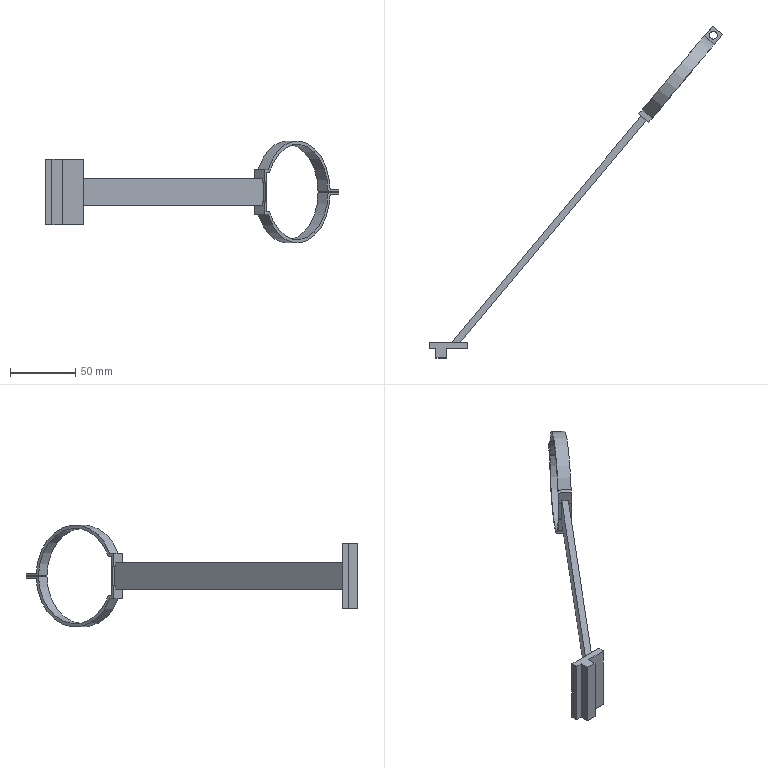Part | SolidWorks | features ICE 7, MirrorPattern 2, BossThin 1, Extrusion 1 | 1 solid | 43 faces | box 224.292 x 253.925 x 78 mm | volume 38659 mm3 | plane 35 | cylinder 8 | commonest cylinder face diameters 6 x4 73 x2 78 x2
STEP:
#1=CARTESIAN_POINT('',(195.164,232.208,2.));
#2=VERTEX_POINT('',#1);
#3=CARTESIAN_POINT('',(201.164,232.208,2.));
#4=VERTEX_POINT('',#3);
#5=CARTESIAN_POINT('',(198.164,232.208,2.));
#6=DIRECTION('',(0.,0.,1.));
#7=DIRECTION('',(1.,0.,0.));
#8=AXIS2_PLACEMENT_3D('',#5,#6,#7);
#9=CIRCLE('',#8,3.);
#10=EDGE_CURVE('',#2,#4,#9,.T.);
#11=ORIENTED_EDGE('',*,*,#10,.T.);
#12=CARTESIAN_POINT('',(201.164,232.208,0.5));
#13=VERTEX_POINT('',#12);
#14=CARTESIAN_POINT('',(201.164,232.208,39.));
#15=DIRECTION('',(0.,0.,-1.));
#16=VECTOR('',#15,1000.);
#17=LINE('',#14,#16);
#18=EDGE_CURVE('',#4,#13,#17,.T.);
#19=ORIENTED_EDGE('',*,*,#18,.T.);
#20=CARTESIAN_POINT('',(195.164,232.208,0.5));
#21=VERTEX_POINT('',#20);
#22=CARTESIAN_POINT('',(198.164,232.208,0.5));
#23=DIRECTION('',(0.,0.,1.));
#24=DIRECTION('',(1.,0.,0.));
#25=AXIS2_PLACEMENT_3D('',#22,#23,#24);
#26=CIRCLE('',#25,3.);
#27=EDGE_CURVE('',#21,#13,#26,.T.);
#28=ORIENTED_EDGE('',*,*,#27,.F.);
#29=CARTESIAN_POINT('',(195.164,232.208,39.));
#30=DIRECTION('',(0.,0.,-1.));
#31=VECTOR('',#30,1000.);
#32=LINE('',#29,#31);
#33=EDGE_CURVE('',#2,#21,#32,.T.);
#34=ORIENTED_EDGE('',*,*,#33,.F.);
#35=EDGE_LOOP('',(#11,#19,#28,#34));
#36=FACE_OUTER_BOUND('',#35,.T.);
#37=CARTESIAN_POINT('',(198.164,232.208,39.));
#38=DIRECTION('',(0.,0.,-1.));
#39=DIRECTION('',(-1.,0.,0.));
#40=AXIS2_PLACEMENT_3D('',#37,#38,#39);
#41=CYLINDRICAL_SURFACE('',#40,3.);
#42=ADVANCED_FACE('',(#36),#41,.F.);
#43=CARTESIAN_POINT('',(201.164,232.208,-0.5));
#44=VERTEX_POINT('',#43);
#45=CARTESIAN_POINT('',(195.164,232.208,-0.5));
#46=VERTEX_POINT('',#45);
#47=CARTESIAN_POINT('',(198.164,232.208,-0.5));
#48=DIRECTION('',(0.,0.,-1.));
#49=DIRECTION('',(-1.,0.,0.));
#50=AXIS2_PLACEMENT_3D('',#47,#48,#49);
#51=CIRCLE('',#50,3.);
#52=EDGE_CURVE('',#44,#46,#51,.T.);
#53=ORIENTED_EDGE('',*,*,#52,.F.);
#54=CARTESIAN_POINT('',(201.164,232.208,-2.));
#55=VERTEX_POINT('',#54);
#56=CARTESIAN_POINT('',(201.164,232.208,39.));
#57=DIRECTION('',(0.,0.,-1.));
#58=VECTOR('',#57,1000.);
#59=LINE('',#56,#58);
#60=EDGE_CURVE('',#44,#55,#59,.T.);
#61=ORIENTED_EDGE('',*,*,#60,.T.);
#62=CARTESIAN_POINT('',(195.164,232.208,-2.));
#63=VERTEX_POINT('',#62);
#64=CARTESIAN_POINT('',(198.164,232.208,-2.));
#65=DIRECTION('',(0.,0.,1.));
#66=DIRECTION('',(1.,0.,0.));
#67=AXIS2_PLACEMENT_3D('',#64,#65,#66);
#68=CIRCLE('',#67,3.);
#69=EDGE_CURVE('',#63,#55,#68,.T.);
#70=ORIENTED_EDGE('',*,*,#69,.F.);
#71=CARTESIAN_POINT('',(195.164,232.208,39.));
#72=DIRECTION('',(0.,0.,-1.));
#73=VECTOR('',#72,1000.);
#74=LINE('',#71,#73);
#75=EDGE_CURVE('',#46,#63,#74,.T.);
#76=ORIENTED_EDGE('',*,*,#75,.F.);
#77=EDGE_LOOP('',(#53,#61,#70,#76));
#78=FACE_OUTER_BOUND('',#77,.T.);
#79=CARTESIAN_POINT('',(198.164,232.208,39.));
#80=DIRECTION('',(0.,0.,-1.));
#81=DIRECTION('',(-1.,0.,0.));
#82=AXIS2_PLACEMENT_3D('',#79,#80,#81);
#83=CYLINDRICAL_SURFACE('',#82,3.);
#84=ADVANCED_FACE('',(#78),#83,.F.);
#85=CARTESIAN_POINT('',(143.02,170.445,10.));
#86=VERTEX_POINT('',#85);
#87=CARTESIAN_POINT('',(-2.232,-2.66,10.));
#88=VERTEX_POINT('',#87);
#89=CARTESIAN_POINT('',(0.,0.,10.));
#90=DIRECTION('',(-0.6428,-0.766,0.));
#91=VECTOR('',#90,1000.);
#92=LINE('',#89,#91);
#93=EDGE_CURVE('',#86,#88,#92,.T.);
#94=ORIENTED_EDGE('',*,*,#93,.T.);
#95=CARTESIAN_POINT('',(4.295,-2.66,10.));
#96=VERTEX_POINT('',#95);
#97=CARTESIAN_POINT('',(4.295,-2.66,10.));
#98=DIRECTION('',(-1.,0.,0.));
#99=VECTOR('',#98,1000.);
#100=LINE('',#97,#99);
#101=EDGE_CURVE('',#96,#88,#100,.T.);
#102=ORIENTED_EDGE('',*,*,#101,.F.);
#103=CARTESIAN_POINT('',(146.85,167.231,10.));
#104=VERTEX_POINT('',#103);
#105=CARTESIAN_POINT('',(4.295,-2.66,10.));
#106=DIRECTION('',(0.6428,0.766,0.));
#107=VECTOR('',#106,1000.);
#108=LINE('',#105,#107);
#109=EDGE_CURVE('',#96,#104,#108,.T.);
#110=ORIENTED_EDGE('',*,*,#109,.T.);
#111=CARTESIAN_POINT('',(143.02,170.445,10.));
#112=DIRECTION('',(0.766,-0.6428,0.));
#113=VECTOR('',#112,1000.);
#114=LINE('',#111,#113);
#115=EDGE_CURVE('',#86,#104,#114,.T.);
#116=ORIENTED_EDGE('',*,*,#115,.F.);
#117=EDGE_LOOP('',(#94,#102,#110,#116));
#118=FACE_OUTER_BOUND('',#117,.T.);
#119=CARTESIAN_POINT('',(0.,0.,10.));
#120=DIRECTION('',(0.,0.,1.));
#121=DIRECTION('',(1.,0.,0.));
#122=AXIS2_PLACEMENT_3D('',#119,#120,#121);
#123=PLANE('',#122);
#124=ADVANCED_FACE('',(#118),#123,.T.);
#125=CARTESIAN_POINT('',(191.045,231.567,-2.));
#126=VERTEX_POINT('',#125);
#127=CARTESIAN_POINT('',(143.606,175.032,-17.5));
#128=VERTEX_POINT('',#127);
#129=CARTESIAN_POINT('',(166.009,201.731,0.));
#130=DIRECTION('',(-0.766,0.6428,0.));
#131=DIRECTION('',(0.,0.,1.));
#132=AXIS2_PLACEMENT_3D('',#129,#130,#131);
#133=CIRCLE('',#132,39.);
#134=EDGE_CURVE('',#126,#128,#133,.T.);
#135=ORIENTED_EDGE('',*,*,#134,.F.);
#136=CARTESIAN_POINT('',(198.705,225.139,-2.));
#137=VERTEX_POINT('',#136);
#138=CARTESIAN_POINT('',(198.705,225.139,-2.));
#139=DIRECTION('',(-0.766,0.6428,0.));
#140=VECTOR('',#139,1000.);
#141=LINE('',#138,#140);
#142=EDGE_CURVE('',#137,#126,#141,.T.);
#143=ORIENTED_EDGE('',*,*,#142,.F.);
#144=CARTESIAN_POINT('',(151.266,168.604,-17.5));
#145=VERTEX_POINT('',#144);
#146=CARTESIAN_POINT('',(173.669,195.303,0.));
#147=DIRECTION('',(-0.766,0.6428,0.));
#148=DIRECTION('',(0.,0.,1.));
#149=AXIS2_PLACEMENT_3D('',#146,#147,#148);
#150=CIRCLE('',#149,39.);
#151=EDGE_CURVE('',#137,#145,#150,.T.);
#152=ORIENTED_EDGE('',*,*,#151,.T.);
#153=CARTESIAN_POINT('',(151.266,168.604,-17.5));
#154=DIRECTION('',(-0.766,0.6428,0.));
#155=VECTOR('',#154,1000.);
#156=LINE('',#153,#155);
#157=EDGE_CURVE('',#145,#128,#156,.T.);
#158=ORIENTED_EDGE('',*,*,#157,.T.);
#159=EDGE_LOOP('',(#135,#143,#152,#158));
#160=FACE_OUTER_BOUND('',#159,.T.);
#161=CARTESIAN_POINT('',(173.669,195.303,0.));
#162=DIRECTION('',(-0.766,0.6428,0.));
#163=DIRECTION('',(-0.6428,-0.766,0.));
#164=AXIS2_PLACEMENT_3D('',#161,#162,#163);
#165=CYLINDRICAL_SURFACE('',#164,39.);
#166=ADVANCED_FACE('',(#160),#165,.T.);
#167=CARTESIAN_POINT('',(198.705,225.139,2.));
#168=VERTEX_POINT('',#167);
#169=CARTESIAN_POINT('',(191.045,231.567,2.));
#170=VERTEX_POINT('',#169);
#171=CARTESIAN_POINT('',(198.705,225.139,2.));
#172=DIRECTION('',(-0.766,0.6428,0.));
#173=VECTOR('',#172,1000.);
#174=LINE('',#171,#173);
#175=EDGE_CURVE('',#168,#170,#174,.T.);
#176=ORIENTED_EDGE('',*,*,#175,.T.);
#177=CARTESIAN_POINT('',(143.606,175.032,17.5));
#178=VERTEX_POINT('',#177);
#179=CARTESIAN_POINT('',(166.009,201.731,0.));
#180=DIRECTION('',(-0.766,0.6428,0.));
#181=DIRECTION('',(0.,0.,1.));
#182=AXIS2_PLACEMENT_3D('',#179,#180,#181);
#183=CIRCLE('',#182,39.);
#184=EDGE_CURVE('',#178,#170,#183,.T.);
#185=ORIENTED_EDGE('',*,*,#184,.F.);
#186=CARTESIAN_POINT('',(151.266,168.604,17.5));
#187=VERTEX_POINT('',#186);
#188=CARTESIAN_POINT('',(151.266,168.604,17.5));
#189=DIRECTION('',(-0.766,0.6428,0.));
#190=VECTOR('',#189,1000.);
#191=LINE('',#188,#190);
#192=EDGE_CURVE('',#187,#178,#191,.T.);
#193=ORIENTED_EDGE('',*,*,#192,.F.);
#194=CARTESIAN_POINT('',(173.669,195.303,0.));
#195=DIRECTION('',(-0.766,0.6428,0.));
#196=DIRECTION('',(0.,0.,1.));
#197=AXIS2_PLACEMENT_3D('',#194,#195,#196);
#198=CIRCLE('',#197,39.);
#199=EDGE_CURVE('',#187,#168,#198,.T.);
#200=ORIENTED_EDGE('',*,*,#199,.T.);
#201=EDGE_LOOP('',(#176,#185,#193,#200));
#202=FACE_OUTER_BOUND('',#201,.T.);
#203=CARTESIAN_POINT('',(173.669,195.303,0.));
#204=DIRECTION('',(-0.766,0.6428,0.));
#205=DIRECTION('',(-0.6428,-0.766,0.));
#206=AXIS2_PLACEMENT_3D('',#203,#204,#205);
#207=CYLINDRICAL_SURFACE('',#206,39.);
#208=ADVANCED_FACE('',(#202),#207,.T.);
#209=CARTESIAN_POINT('',(144.62,176.24,15.));
#210=VERTEX_POINT('',#209);
#211=CARTESIAN_POINT('',(189.468,229.689,0.5));
#212=VERTEX_POINT('',#211);
#213=CARTESIAN_POINT('',(166.009,201.731,0.));
#214=DIRECTION('',(-0.766,0.6428,0.));
#215=DIRECTION('',(-0.6428,-0.766,0.));
#216=AXIS2_PLACEMENT_3D('',#213,#214,#215);
#217=CIRCLE('',#216,36.5);
#218=EDGE_CURVE('',#210,#212,#217,.T.);
#219=ORIENTED_EDGE('',*,*,#218,.T.);
#220=CARTESIAN_POINT('',(197.129,223.261,0.5));
#221=VERTEX_POINT('',#220);
#222=CARTESIAN_POINT('',(197.129,223.261,0.5));
#223=DIRECTION('',(0.766,-0.6428,0.));
#224=VECTOR('',#223,1000.);
#225=LINE('',#222,#224);
#226=EDGE_CURVE('',#212,#221,#225,.T.);
#227=ORIENTED_EDGE('',*,*,#226,.T.);
#228=CARTESIAN_POINT('',(152.28,169.813,15.));
#229=VERTEX_POINT('',#228);
#230=CARTESIAN_POINT('',(173.669,195.303,0.));
#231=DIRECTION('',(-0.766,0.6428,0.));
#232=DIRECTION('',(-0.6428,-0.766,0.));
#233=AXIS2_PLACEMENT_3D('',#230,#231,#232);
#234=CIRCLE('',#233,36.5);
#235=EDGE_CURVE('',#229,#221,#234,.T.);
#236=ORIENTED_EDGE('',*,*,#235,.F.);
#237=CARTESIAN_POINT('',(152.28,169.813,15.));
#238=DIRECTION('',(-0.766,0.6428,0.));
#239=VECTOR('',#238,1000.);
#240=LINE('',#237,#239);
#241=EDGE_CURVE('',#229,#210,#240,.T.);
#242=ORIENTED_EDGE('',*,*,#241,.T.);
#243=EDGE_LOOP('',(#219,#227,#236,#242));
#244=FACE_OUTER_BOUND('',#243,.T.);
#245=CARTESIAN_POINT('',(173.669,195.303,0.));
#246=DIRECTION('',(-0.766,0.6428,0.));
#247=DIRECTION('',(-0.6428,-0.766,0.));
#248=AXIS2_PLACEMENT_3D('',#245,#246,#247);
#249=CYLINDRICAL_SURFACE('',#248,36.5);
#250=ADVANCED_FACE('',(#244),#249,.F.);
#251=CARTESIAN_POINT('',(-6.128,-7.66,25.));
#252=VERTEX_POINT('',#251);
#253=CARTESIAN_POINT('',(10.,-7.66,25.));
#254=VERTEX_POINT('',#253);
#255=CARTESIAN_POINT('',(-6.428,-7.66,25.));
#256=DIRECTION('',(1.,0.,0.));
#257=VECTOR('',#256,1000.);
#258=LINE('',#255,#257);
#259=EDGE_CURVE('',#252,#254,#258,.T.);
#260=ORIENTED_EDGE('',*,*,#259,.F.);
#261=CARTESIAN_POINT('',(-6.128,-7.66,-25.));
#262=VERTEX_POINT('',#261);
#263=CARTESIAN_POINT('',(-6.128,-7.66,45.723));
#264=DIRECTION('',(0.,0.,-1.));
#265=VECTOR('',#264,1000.);
#266=LINE('',#263,#265);
#267=EDGE_CURVE('',#252,#262,#266,.T.);
#268=ORIENTED_EDGE('',*,*,#267,.T.);
#269=CARTESIAN_POINT('',(10.,-7.66,-25.));
#270=VERTEX_POINT('',#269);
#271=CARTESIAN_POINT('',(-6.428,-7.66,-25.));
#272=DIRECTION('',(1.,0.,0.));
#273=VECTOR('',#272,1000.);
#274=LINE('',#271,#273);
#275=EDGE_CURVE('',#262,#270,#274,.T.);
#276=ORIENTED_EDGE('',*,*,#275,.T.);
#277=CARTESIAN_POINT('',(10.,-7.66,10.));
#278=DIRECTION('',(0.,0.,-1.));
#279=VECTOR('',#278,1000.);
#280=LINE('',#277,#279);
#281=EDGE_CURVE('',#254,#270,#280,.T.);
#282=ORIENTED_EDGE('',*,*,#281,.F.);
#283=EDGE_LOOP('',(#260,#268,#276,#282));
#284=FACE_OUTER_BOUND('',#283,.T.);
#285=CARTESIAN_POINT('',(-6.428,-7.66,10.));
#286=DIRECTION('',(0.,1.,0.));
#287=DIRECTION('',(0.,0.,1.));
#288=AXIS2_PLACEMENT_3D('',#285,#286,#287);
#289=PLANE('',#288);
#290=ADVANCED_FACE('',(#284),#289,.F.);
#291=CARTESIAN_POINT('',(-2.232,-2.66,-10.));
#292=VERTEX_POINT('',#291);
#293=CARTESIAN_POINT('',(-2.232,-2.66,45.723));
#294=DIRECTION('',(0.,0.,-1.));
#295=VECTOR('',#294,1000.);
#296=LINE('',#293,#295);
#297=EDGE_CURVE('',#88,#292,#296,.T.);
#298=ORIENTED_EDGE('',*,*,#297,.T.);
#299=CARTESIAN_POINT('',(4.295,-2.66,-10.));
#300=VERTEX_POINT('',#299);
#301=CARTESIAN_POINT('',(10.,-2.66,-10.));
#302=DIRECTION('',(-1.,0.,0.));
#303=VECTOR('',#302,1000.);
#304=LINE('',#301,#303);
#305=EDGE_CURVE('',#300,#292,#304,.T.);
#306=ORIENTED_EDGE('',*,*,#305,.F.);
#307=CARTESIAN_POINT('',(4.295,-2.66,10.));
#308=DIRECTION('',(0.,0.,-1.));
#309=VECTOR('',#308,1000.);
#310=LINE('',#307,#309);
#311=EDGE_CURVE('',#96,#300,#310,.T.);
#312=ORIENTED_EDGE('',*,*,#311,.F.);
#313=ORIENTED_EDGE('',*,*,#101,.T.);
#314=EDGE_LOOP('',(#298,#306,#312,#313));
#315=FACE_BOUND('',#314,.T.);
#316=CARTESIAN_POINT('',(10.,-2.66,-25.));
#317=VERTEX_POINT('',#316);
#318=CARTESIAN_POINT('',(-19.128,-2.66,-25.));
#319=VERTEX_POINT('',#318);
#320=CARTESIAN_POINT('',(4.295,-2.66,-25.));
#321=DIRECTION('',(-1.,0.,0.));
#322=VECTOR('',#321,1000.);
#323=LINE('',#320,#322);
#324=EDGE_CURVE('',#317,#319,#323,.T.);
#325=ORIENTED_EDGE('',*,*,#324,.T.);
#326=CARTESIAN_POINT('',(-19.128,-2.66,25.));
#327=VERTEX_POINT('',#326);
#328=CARTESIAN_POINT('',(-19.128,-2.66,45.723));
#329=DIRECTION('',(0.,0.,-1.));
#330=VECTOR('',#329,1000.);
#331=LINE('',#328,#330);
#332=EDGE_CURVE('',#327,#319,#331,.T.);
#333=ORIENTED_EDGE('',*,*,#332,.F.);
#334=CARTESIAN_POINT('',(10.,-2.66,25.));
#335=VERTEX_POINT('',#334);
#336=CARTESIAN_POINT('',(10.,-2.66,25.));
#337=DIRECTION('',(-1.,0.,0.));
#338=VECTOR('',#337,1000.);
#339=LINE('',#336,#338);
#340=EDGE_CURVE('',#335,#327,#339,.T.);
#341=ORIENTED_EDGE('',*,*,#340,.F.);
#342=CARTESIAN_POINT('',(10.,-2.66,10.));
#343=DIRECTION('',(0.,0.,-1.));
#344=VECTOR('',#343,1000.);
#345=LINE('',#342,#344);
#346=EDGE_CURVE('',#335,#317,#345,.T.);
#347=ORIENTED_EDGE('',*,*,#346,.T.);
#348=EDGE_LOOP('',(#325,#333,#341,#347));
#349=FACE_OUTER_BOUND('',#348,.T.);
#350=CARTESIAN_POINT('',(30.,-2.66,10.));
#351=DIRECTION('',(0.,-1.,0.));
#352=DIRECTION('',(1.,0.,0.));
#353=AXIS2_PLACEMENT_3D('',#350,#351,#352);
#354=PLANE('',#353);
#355=ADVANCED_FACE('',(#315,#349),#354,.F.);
#356=CARTESIAN_POINT('',(147.493,167.997,7.5));
#357=VERTEX_POINT('',#356);
#358=CARTESIAN_POINT('',(146.85,167.231,7.5));
#359=VERTEX_POINT('',#358);
#360=CARTESIAN_POINT('',(149.1,169.912,7.5));
#361=DIRECTION('',(-0.6428,-0.766,0.));
#362=VECTOR('',#361,1000.);
#363=LINE('',#360,#362);
#364=EDGE_CURVE('',#357,#359,#363,.T.);
#365=ORIENTED_EDGE('',*,*,#364,.T.);
#366=CARTESIAN_POINT('',(146.85,167.231,10.));
#367=DIRECTION('',(0.,0.,1.));
#368=VECTOR('',#367,1000.);
#369=LINE('',#366,#368);
#370=EDGE_CURVE('',#359,#104,#369,.T.);
#371=ORIENTED_EDGE('',*,*,#370,.T.);
#372=ORIENTED_EDGE('',*,*,#109,.F.);
#373=ORIENTED_EDGE('',*,*,#311,.T.);
#374=CARTESIAN_POINT('',(146.85,167.231,-10.));
#375=VERTEX_POINT('',#374);
#376=CARTESIAN_POINT('',(149.1,169.912,-10.));
#377=DIRECTION('',(0.6428,0.766,0.));
#378=VECTOR('',#377,1000.);
#379=LINE('',#376,#378);
#380=EDGE_CURVE('',#300,#375,#379,.T.);
#381=ORIENTED_EDGE('',*,*,#380,.T.);
#382=CARTESIAN_POINT('',(146.85,167.231,-7.5));
#383=VERTEX_POINT('',#382);
#384=CARTESIAN_POINT('',(146.85,167.231,10.));
#385=DIRECTION('',(0.,0.,1.));
#386=VECTOR('',#385,1000.);
#387=LINE('',#384,#386);
#388=EDGE_CURVE('',#375,#383,#387,.T.);
#389=ORIENTED_EDGE('',*,*,#388,.T.);
#390=CARTESIAN_POINT('',(147.493,167.997,-7.5));
#391=VERTEX_POINT('',#390);
#392=CARTESIAN_POINT('',(149.1,169.912,-7.5));
#393=DIRECTION('',(0.6428,0.766,0.));
#394=VECTOR('',#393,1000.);
#395=LINE('',#392,#394);
#396=EDGE_CURVE('',#383,#391,#395,.T.);
#397=ORIENTED_EDGE('',*,*,#396,.T.);
#398=CARTESIAN_POINT('',(147.493,167.997,10.));
#399=DIRECTION('',(0.,0.,1.));
#400=VECTOR('',#399,1000.);
#401=LINE('',#398,#400);
#402=EDGE_CURVE('',#391,#357,#401,.T.);
#403=ORIENTED_EDGE('',*,*,#402,.T.);
#404=EDGE_LOOP('',(#365,#371,#372,#373,#381,#389,#397,#403));
#405=FACE_OUTER_BOUND('',#404,.T.);
#406=CARTESIAN_POINT('',(149.1,169.912,10.));
#407=DIRECTION('',(-0.766,0.6428,0.));
#408=DIRECTION('',(-0.6428,-0.766,0.));
#409=AXIS2_PLACEMENT_3D('',#406,#407,#408);
#410=PLANE('',#409);
#411=ADVANCED_FACE('',(#405),#410,.F.);
#412=CARTESIAN_POINT('',(143.02,170.445,-10.));
#413=VERTEX_POINT('',#412);
#414=CARTESIAN_POINT('',(0.,0.,-10.));
#415=DIRECTION('',(-0.6428,-0.766,0.));
#416=VECTOR('',#415,1000.);
#417=LINE('',#414,#416);
#418=EDGE_CURVE('',#413,#292,#417,.T.);
#419=ORIENTED_EDGE('',*,*,#418,.T.);
#420=ORIENTED_EDGE('',*,*,#297,.F.);
#421=ORIENTED_EDGE('',*,*,#93,.F.);
#422=CARTESIAN_POINT('',(143.02,170.445,7.5));
#423=VERTEX_POINT('',#422);
#424=CARTESIAN_POINT('',(143.02,170.445,10.));
#425=DIRECTION('',(0.,0.,-1.));
#426=VECTOR('',#425,1000.);
#427=LINE('',#424,#426);
#428=EDGE_CURVE('',#86,#423,#427,.T.);
#429=ORIENTED_EDGE('',*,*,#428,.T.);
#430=CARTESIAN_POINT('',(143.663,171.211,7.5));
#431=VERTEX_POINT('',#430);
#432=CARTESIAN_POINT('',(0.,0.,7.5));
#433=DIRECTION('',(0.6428,0.766,0.));
#434=VECTOR('',#433,1000.);
#435=LINE('',#432,#434);
#436=EDGE_CURVE('',#423,#431,#435,.T.);
#437=ORIENTED_EDGE('',*,*,#436,.T.);
#438=CARTESIAN_POINT('',(143.663,171.211,-7.5));
#439=VERTEX_POINT('',#438);
#440=CARTESIAN_POINT('',(143.663,171.211,10.));
#441=DIRECTION('',(0.,0.,-1.));
#442=VECTOR('',#441,1000.);
#443=LINE('',#440,#442);
#444=EDGE_CURVE('',#431,#439,#443,.T.);
#445=ORIENTED_EDGE('',*,*,#444,.T.);
#446=CARTESIAN_POINT('',(143.02,170.445,-7.5));
#447=VERTEX_POINT('',#446);
#448=CARTESIAN_POINT('',(0.,0.,-7.5));
#449=DIRECTION('',(-0.6428,-0.766,0.));
#450=VECTOR('',#449,1000.);
#451=LINE('',#448,#450);
#452=EDGE_CURVE('',#439,#447,#451,.T.);
#453=ORIENTED_EDGE('',*,*,#452,.T.);
#454=CARTESIAN_POINT('',(143.02,170.445,10.));
#455=DIRECTION('',(0.,0.,-1.));
#456=VECTOR('',#455,1000.);
#457=LINE('',#454,#456);
#458=EDGE_CURVE('',#447,#413,#457,.T.);
#459=ORIENTED_EDGE('',*,*,#458,.T.);
#460=EDGE_LOOP('',(#419,#420,#421,#429,#437,#445,#453,#459));
#461=FACE_OUTER_BOUND('',#460,.T.);
#462=CARTESIAN_POINT('',(0.,0.,10.));
#463=DIRECTION('',(0.766,-0.6428,0.));
#464=DIRECTION('',(0.6428,0.766,0.));
#465=AXIS2_PLACEMENT_3D('',#462,#463,#464);
#466=PLANE('',#465);
#467=ADVANCED_FACE('',(#461),#466,.F.);
#468=ORIENTED_EDGE('',*,*,#380,.F.);
#469=ORIENTED_EDGE('',*,*,#305,.T.);
#470=ORIENTED_EDGE('',*,*,#418,.F.);
#471=CARTESIAN_POINT('',(143.02,170.445,-10.));
#472=DIRECTION('',(0.766,-0.6428,0.));
#473=VECTOR('',#472,1000.);
#474=LINE('',#471,#473);
#475=EDGE_CURVE('',#413,#375,#474,.T.);
#476=ORIENTED_EDGE('',*,*,#475,.T.);
#477=EDGE_LOOP('',(#468,#469,#470,#476));
#478=FACE_OUTER_BOUND('',#477,.T.);
#479=CARTESIAN_POINT('',(0.,0.,-10.));
#480=DIRECTION('',(0.,0.,1.));
#481=DIRECTION('',(1.,0.,0.));
#482=AXIS2_PLACEMENT_3D('',#479,#480,#481);
#483=PLANE('',#482);
#484=ADVANCED_FACE('',(#478),#483,.F.);
#485=ORIENTED_EDGE('',*,*,#364,.F.);
#486=CARTESIAN_POINT('',(149.408,166.39,7.5));
#487=VERTEX_POINT('',#486);
#488=CARTESIAN_POINT('',(149.408,166.39,7.5));
#489=DIRECTION('',(-0.766,0.6428,0.));
#490=VECTOR('',#489,1000.);
#491=LINE('',#488,#490);
#492=EDGE_CURVE('',#487,#357,#491,.T.);
#493=ORIENTED_EDGE('',*,*,#492,.F.);
#494=CARTESIAN_POINT('',(148.766,165.624,7.5));
#495=VERTEX_POINT('',#494);
#496=CARTESIAN_POINT('',(5.745,-4.821,7.5));
#497=DIRECTION('',(-0.6428,-0.766,0.));
#498=VECTOR('',#497,1000.);
#499=LINE('',#496,#498);
#500=EDGE_CURVE('',#487,#495,#499,.T.);
#501=ORIENTED_EDGE('',*,*,#500,.T.);
#502=CARTESIAN_POINT('',(148.766,165.624,7.5));
#503=DIRECTION('',(-0.766,0.6428,0.));
#504=VECTOR('',#503,1000.);
#505=LINE('',#502,#504);
#506=EDGE_CURVE('',#495,#359,#505,.T.);
#507=ORIENTED_EDGE('',*,*,#506,.T.);
#508=EDGE_LOOP('',(#485,#493,#501,#507));
#509=FACE_OUTER_BOUND('',#508,.T.);
#510=CARTESIAN_POINT('',(5.745,-4.821,7.5));
#511=DIRECTION('',(0.,0.,-1.));
#512=DIRECTION('',(-1.,0.,0.));
#513=AXIS2_PLACEMENT_3D('',#510,#511,#512);
#514=PLANE('',#513);
#515=ADVANCED_FACE('',(#509),#514,.T.);
#516=ORIENTED_EDGE('',*,*,#436,.F.);
#517=CARTESIAN_POINT('',(141.105,172.052,7.5));
#518=VERTEX_POINT('',#517);
#519=CARTESIAN_POINT('',(148.766,165.624,7.5));
#520=DIRECTION('',(-0.766,0.6428,0.));
#521=VECTOR('',#520,1000.);
#522=LINE('',#519,#521);
#523=EDGE_CURVE('',#423,#518,#522,.T.);
#524=ORIENTED_EDGE('',*,*,#523,.T.);
#525=CARTESIAN_POINT('',(141.748,172.818,7.5));
#526=VERTEX_POINT('',#525);
#527=CARTESIAN_POINT('',(-1.915,1.607,7.5));
#528=DIRECTION('',(-0.6428,-0.766,0.));
#529=VECTOR('',#528,1000.);
#530=LINE('',#527,#529);
#531=EDGE_CURVE('',#526,#518,#530,.T.);
#532=ORIENTED_EDGE('',*,*,#531,.F.);
#533=CARTESIAN_POINT('',(149.408,166.39,7.5));
#534=DIRECTION('',(-0.766,0.6428,0.));
#535=VECTOR('',#534,1000.);
#536=LINE('',#533,#535);
#537=EDGE_CURVE('',#431,#526,#536,.T.);
#538=ORIENTED_EDGE('',*,*,#537,.F.);
#539=EDGE_LOOP('',(#516,#524,#532,#538));
#540=FACE_OUTER_BOUND('',#539,.T.);
#541=CARTESIAN_POINT('',(5.745,-4.821,7.5));
#542=DIRECTION('',(0.,0.,-1.));
#543=DIRECTION('',(-1.,0.,0.));
#544=AXIS2_PLACEMENT_3D('',#541,#542,#543);
#545=PLANE('',#544);
#546=ADVANCED_FACE('',(#540),#545,.T.);
#547=ORIENTED_EDGE('',*,*,#402,.F.);
#548=CARTESIAN_POINT('',(149.408,166.39,-7.5));
#549=VERTEX_POINT('',#548);
#550=CARTESIAN_POINT('',(149.408,166.39,-7.5));
#551=DIRECTION('',(-0.766,0.6428,0.));
#552=VECTOR('',#551,1000.);
#553=LINE('',#550,#552);
#554=EDGE_CURVE('',#549,#391,#553,.T.);
#555=ORIENTED_EDGE('',*,*,#554,.F.);
#556=CARTESIAN_POINT('',(149.408,166.39,0.));
#557=DIRECTION('',(0.,0.,1.));
#558=VECTOR('',#557,1000.);
#559=LINE('',#556,#558);
#560=EDGE_CURVE('',#549,#487,#559,.T.);
#561=ORIENTED_EDGE('',*,*,#560,.T.);
#562=ORIENTED_EDGE('',*,*,#492,.T.);
#563=EDGE_LOOP('',(#547,#555,#561,#562));
#564=FACE_OUTER_BOUND('',#563,.T.);
#565=CARTESIAN_POINT('',(149.408,166.39,0.));
#566=DIRECTION('',(-0.6428,-0.766,0.));
#567=DIRECTION('',(0.766,-0.6428,0.));
#568=AXIS2_PLACEMENT_3D('',#565,#566,#567);
#569=PLANE('',#568);
#570=ADVANCED_FACE('',(#564),#569,.T.);
#571=ORIENTED_EDGE('',*,*,#444,.F.);
#572=ORIENTED_EDGE('',*,*,#537,.T.);
#573=CARTESIAN_POINT('',(141.748,172.818,-7.5));
#574=VERTEX_POINT('',#573);
#575=CARTESIAN_POINT('',(141.748,172.818,0.));
#576=DIRECTION('',(0.,0.,1.));
#577=VECTOR('',#576,1000.);
#578=LINE('',#575,#577);
#579=EDGE_CURVE('',#574,#526,#578,.T.);
#580=ORIENTED_EDGE('',*,*,#579,.F.);
#581=CARTESIAN_POINT('',(149.408,166.39,-7.5));
#582=DIRECTION('',(-0.766,0.6428,0.));
#583=VECTOR('',#582,1000.);
#584=LINE('',#581,#583);
#585=EDGE_CURVE('',#439,#574,#584,.T.);
#586=ORIENTED_EDGE('',*,*,#585,.F.);
#587=EDGE_LOOP('',(#571,#572,#580,#586));
#588=FACE_OUTER_BOUND('',#587,.T.);
#589=CARTESIAN_POINT('',(149.408,166.39,0.));
#590=DIRECTION('',(-0.6428,-0.766,0.));
#591=DIRECTION('',(0.766,-0.6428,0.));
#592=AXIS2_PLACEMENT_3D('',#589,#590,#591);
#593=PLANE('',#592);
#594=ADVANCED_FACE('',(#588),#593,.T.);
#595=ORIENTED_EDGE('',*,*,#396,.F.);
#596=CARTESIAN_POINT('',(148.766,165.624,-7.5));
#597=VERTEX_POINT('',#596);
#598=CARTESIAN_POINT('',(148.766,165.624,-7.5));
#599=DIRECTION('',(-0.766,0.6428,0.));
#600=VECTOR('',#599,1000.);
#601=LINE('',#598,#600);
#602=EDGE_CURVE('',#597,#383,#601,.T.);
#603=ORIENTED_EDGE('',*,*,#602,.F.);
#604=CARTESIAN_POINT('',(5.745,-4.821,-7.5));
#605=DIRECTION('',(0.6428,0.766,0.));
#606=VECTOR('',#605,1000.);
#607=LINE('',#604,#606);
#608=EDGE_CURVE('',#597,#549,#607,.T.);
#609=ORIENTED_EDGE('',*,*,#608,.T.);
#610=ORIENTED_EDGE('',*,*,#554,.T.);
#611=EDGE_LOOP('',(#595,#603,#609,#610));
#612=FACE_OUTER_BOUND('',#611,.T.);
#613=CARTESIAN_POINT('',(5.745,-4.821,-7.5));
#614=DIRECTION('',(0.,0.,1.));
#615=DIRECTION('',(1.,0.,0.));
#616=AXIS2_PLACEMENT_3D('',#613,#614,#615);
#617=PLANE('',#616);
#618=ADVANCED_FACE('',(#612),#617,.T.);
#619=ORIENTED_EDGE('',*,*,#452,.F.);
#620=ORIENTED_EDGE('',*,*,#585,.T.);
#621=CARTESIAN_POINT('',(141.105,172.052,-7.5));
#622=VERTEX_POINT('',#621);
#623=CARTESIAN_POINT('',(-1.915,1.607,-7.5));
#624=DIRECTION('',(0.6428,0.766,0.));
#625=VECTOR('',#624,1000.);
#626=LINE('',#623,#625);
#627=EDGE_CURVE('',#622,#574,#626,.T.);
#628=ORIENTED_EDGE('',*,*,#627,.F.);
#629=CARTESIAN_POINT('',(148.766,165.624,-7.5));
#630=DIRECTION('',(-0.766,0.6428,0.));
#631=VECTOR('',#630,1000.);
#632=LINE('',#629,#631);
#633=EDGE_CURVE('',#447,#622,#632,.T.);
#634=ORIENTED_EDGE('',*,*,#633,.F.);
#635=EDGE_LOOP('',(#619,#620,#628,#634));
#636=FACE_OUTER_BOUND('',#635,.T.);
#637=CARTESIAN_POINT('',(5.745,-4.821,-7.5));
#638=DIRECTION('',(0.,0.,1.));
#639=DIRECTION('',(1.,0.,0.));
#640=AXIS2_PLACEMENT_3D('',#637,#638,#639);
#641=PLANE('',#640);
#642=ADVANCED_FACE('',(#636),#641,.T.);
#643=ORIENTED_EDGE('',*,*,#370,.F.);
#644=ORIENTED_EDGE('',*,*,#506,.F.);
#645=CARTESIAN_POINT('',(148.766,165.624,17.5));
#646=VERTEX_POINT('',#645);
#647=CARTESIAN_POINT('',(148.766,165.624,0.));
#648=DIRECTION('',(0.,0.,1.));
#649=VECTOR('',#648,1000.);
#650=LINE('',#647,#649);
#651=EDGE_CURVE('',#495,#646,#650,.T.);
#652=ORIENTED_EDGE('',*,*,#651,.T.);
#653=CARTESIAN_POINT('',(141.105,172.052,17.5));
#654=VERTEX_POINT('',#653);
#655=CARTESIAN_POINT('',(148.766,165.624,17.5));
#656=DIRECTION('',(-0.766,0.6428,0.));
#657=VECTOR('',#656,1000.);
#658=LINE('',#655,#657);
#659=EDGE_CURVE('',#646,#654,#658,.T.);
#660=ORIENTED_EDGE('',*,*,#659,.T.);
#661=CARTESIAN_POINT('',(141.105,172.052,0.));
#662=DIRECTION('',(0.,0.,1.));
#663=VECTOR('',#662,1000.);
#664=LINE('',#661,#663);
#665=EDGE_CURVE('',#518,#654,#664,.T.);
#666=ORIENTED_EDGE('',*,*,#665,.F.);
#667=ORIENTED_EDGE('',*,*,#523,.F.);
#668=ORIENTED_EDGE('',*,*,#428,.F.);
#669=ORIENTED_EDGE('',*,*,#115,.T.);
#670=EDGE_LOOP('',(#643,#644,#652,#660,#666,#667,#668,#669));
#671=FACE_OUTER_BOUND('',#670,.T.);
#672=CARTESIAN_POINT('',(148.766,165.624,0.));
#673=DIRECTION('',(-0.6428,-0.766,0.));
#674=DIRECTION('',(0.766,-0.6428,0.));
#675=AXIS2_PLACEMENT_3D('',#672,#673,#674);
#676=PLANE('',#675);
#677=ADVANCED_FACE('',(#671),#676,.T.);
#678=ORIENTED_EDGE('',*,*,#388,.F.);
#679=ORIENTED_EDGE('',*,*,#475,.F.);
#680=ORIENTED_EDGE('',*,*,#458,.F.);
#681=ORIENTED_EDGE('',*,*,#633,.T.);
#682=CARTESIAN_POINT('',(141.105,172.052,-17.5));
#683=VERTEX_POINT('',#682);
#684=CARTESIAN_POINT('',(141.105,172.052,0.));
#685=DIRECTION('',(0.,0.,1.));
#686=VECTOR('',#685,1000.);
#687=LINE('',#684,#686);
#688=EDGE_CURVE('',#683,#622,#687,.T.);
#689=ORIENTED_EDGE('',*,*,#688,.F.);
#690=CARTESIAN_POINT('',(148.766,165.624,-17.5));
#691=VERTEX_POINT('',#690);
#692=CARTESIAN_POINT('',(148.766,165.624,-17.5));
#693=DIRECTION('',(-0.766,0.6428,0.));
#694=VECTOR('',#693,1000.);
#695=LINE('',#692,#694);
#696=EDGE_CURVE('',#691,#683,#695,.T.);
#697=ORIENTED_EDGE('',*,*,#696,.F.);
#698=CARTESIAN_POINT('',(148.766,165.624,0.));
#699=DIRECTION('',(0.,0.,1.));
#700=VECTOR('',#699,1000.);
#701=LINE('',#698,#700);
#702=EDGE_CURVE('',#691,#597,#701,.T.);
#703=ORIENTED_EDGE('',*,*,#702,.T.);
#704=ORIENTED_EDGE('',*,*,#602,.T.);
#705=EDGE_LOOP('',(#678,#679,#680,#681,#689,#697,#703,#704));
#706=FACE_OUTER_BOUND('',#705,.T.);
#707=CARTESIAN_POINT('',(148.766,165.624,0.));
#708=DIRECTION('',(-0.6428,-0.766,0.));
#709=DIRECTION('',(0.766,-0.6428,0.));
#710=AXIS2_PLACEMENT_3D('',#707,#708,#709);
#711=PLANE('',#710);
#712=ADVANCED_FACE('',(#706),#711,.T.);
#713=ORIENTED_EDGE('',*,*,#192,.T.);
#714=CARTESIAN_POINT('',(-1.915,1.607,17.5));
#715=DIRECTION('',(0.6428,0.766,0.));
#716=VECTOR('',#715,1000.);
#717=LINE('',#714,#716);
#718=EDGE_CURVE('',#654,#178,#717,.T.);
#719=ORIENTED_EDGE('',*,*,#718,.F.);
#720=ORIENTED_EDGE('',*,*,#659,.F.);
#721=CARTESIAN_POINT('',(5.745,-4.821,17.5));
#722=DIRECTION('',(0.6428,0.766,0.));
#723=VECTOR('',#722,1000.);
#724=LINE('',#721,#723);
#725=EDGE_CURVE('',#646,#187,#724,.T.);
#726=ORIENTED_EDGE('',*,*,#725,.T.);
#727=EDGE_LOOP('',(#713,#719,#720,#726));
#728=FACE_OUTER_BOUND('',#727,.T.);
#729=CARTESIAN_POINT('',(5.745,-4.821,17.5));
#730=DIRECTION('',(0.,0.,1.));
#731=DIRECTION('',(1.,0.,0.));
#732=AXIS2_PLACEMENT_3D('',#729,#730,#731);
#733=PLANE('',#732);
#734=ADVANCED_FACE('',(#728),#733,.T.);
#735=ORIENTED_EDGE('',*,*,#696,.T.);
#736=CARTESIAN_POINT('',(-1.915,1.607,-17.5));
#737=DIRECTION('',(-0.6428,-0.766,0.));
#738=VECTOR('',#737,1000.);
#739=LINE('',#736,#738);
#740=EDGE_CURVE('',#128,#683,#739,.T.);
#741=ORIENTED_EDGE('',*,*,#740,.F.);
#742=ORIENTED_EDGE('',*,*,#157,.F.);
#743=CARTESIAN_POINT('',(5.745,-4.821,-17.5));
#744=DIRECTION('',(-0.6428,-0.766,0.));
#745=VECTOR('',#744,1000.);
#746=LINE('',#743,#745);
#747=EDGE_CURVE('',#145,#691,#746,.T.);
#748=ORIENTED_EDGE('',*,*,#747,.T.);
#749=EDGE_LOOP('',(#735,#741,#742,#748));
#750=FACE_OUTER_BOUND('',#749,.T.);
#751=CARTESIAN_POINT('',(5.745,-4.821,-17.5));
#752=DIRECTION('',(0.,0.,-1.));
#753=DIRECTION('',(-1.,0.,0.));
#754=AXIS2_PLACEMENT_3D('',#751,#752,#753);
#755=PLANE('',#754);
#756=ADVANCED_FACE('',(#750),#755,.T.);
#757=ORIENTED_EDGE('',*,*,#235,.T.);
#758=CARTESIAN_POINT('',(205.164,232.837,0.5));
#759=VERTEX_POINT('',#758);
#760=CARTESIAN_POINT('',(173.669,195.303,0.5));
#761=DIRECTION('',(0.6428,0.766,0.));
#762=VECTOR('',#761,1000.);
#763=LINE('',#760,#762);
#764=EDGE_CURVE('',#221,#759,#763,.T.);
#765=ORIENTED_EDGE('',*,*,#764,.T.);
#766=CARTESIAN_POINT('',(205.164,232.837,2.));
#767=VERTEX_POINT('',#766);
#768=CARTESIAN_POINT('',(205.164,232.837,0.5));
#769=DIRECTION('',(0.,0.,-1.));
#770=VECTOR('',#769,1000.);
#771=LINE('',#768,#770);
#772=EDGE_CURVE('',#767,#759,#771,.T.);
#773=ORIENTED_EDGE('',*,*,#772,.F.);
#774=CARTESIAN_POINT('',(-0.6838,-12.483,2.));
#775=DIRECTION('',(0.6428,0.766,0.));
#776=VECTOR('',#775,1000.);
#777=LINE('',#774,#776);
#778=EDGE_CURVE('',#168,#767,#777,.T.);
#779=ORIENTED_EDGE('',*,*,#778,.F.);
#780=ORIENTED_EDGE('',*,*,#199,.F.);
#781=ORIENTED_EDGE('',*,*,#725,.F.);
#782=ORIENTED_EDGE('',*,*,#651,.F.);
#783=ORIENTED_EDGE('',*,*,#500,.F.);
#784=ORIENTED_EDGE('',*,*,#560,.F.);
#785=ORIENTED_EDGE('',*,*,#608,.F.);
#786=ORIENTED_EDGE('',*,*,#702,.F.);
#787=ORIENTED_EDGE('',*,*,#747,.F.);
#788=ORIENTED_EDGE('',*,*,#151,.F.);
#789=CARTESIAN_POINT('',(205.164,232.837,-2.));
#790=VERTEX_POINT('',#789);
#791=CARTESIAN_POINT('',(-0.6838,-12.483,-2.));
#792=DIRECTION('',(0.6428,0.766,0.));
#793=VECTOR('',#792,1000.);
#794=LINE('',#791,#793);
#795=EDGE_CURVE('',#137,#790,#794,.T.);
#796=ORIENTED_EDGE('',*,*,#795,.T.);
#797=CARTESIAN_POINT('',(205.164,232.837,-0.5));
#798=VERTEX_POINT('',#797);
#799=CARTESIAN_POINT('',(205.164,232.837,-0.5));
#800=DIRECTION('',(0.,0.,1.));
#801=VECTOR('',#800,1000.);
#802=LINE('',#799,#801);
#803=EDGE_CURVE('',#790,#798,#802,.T.);
#804=ORIENTED_EDGE('',*,*,#803,.T.);
#805=CARTESIAN_POINT('',(197.129,223.261,-0.5));
#806=VERTEX_POINT('',#805);
#807=CARTESIAN_POINT('',(173.669,195.303,-0.5));
#808=DIRECTION('',(-0.6428,-0.766,0.));
#809=VECTOR('',#808,1000.);
#810=LINE('',#807,#809);
#811=EDGE_CURVE('',#798,#806,#810,.T.);
#812=ORIENTED_EDGE('',*,*,#811,.T.);
#813=CARTESIAN_POINT('',(152.28,169.813,-15.));
#814=VERTEX_POINT('',#813);
#815=CARTESIAN_POINT('',(173.669,195.303,0.));
#816=DIRECTION('',(-0.766,0.6428,0.));
#817=DIRECTION('',(-0.6428,-0.766,0.));
#818=AXIS2_PLACEMENT_3D('',#815,#816,#817);
#819=CIRCLE('',#818,36.5);
#820=EDGE_CURVE('',#806,#814,#819,.T.);
#821=ORIENTED_EDGE('',*,*,#820,.T.);
#822=CARTESIAN_POINT('',(150.373,167.539,-15.));
#823=VERTEX_POINT('',#822);
#824=CARTESIAN_POINT('',(5.745,-4.821,-15.));
#825=DIRECTION('',(-0.6428,-0.766,0.));
#826=VECTOR('',#825,1000.);
#827=LINE('',#824,#826);
#828=EDGE_CURVE('',#814,#823,#827,.T.);
#829=ORIENTED_EDGE('',*,*,#828,.T.);
#830=CARTESIAN_POINT('',(150.373,167.539,15.));
#831=VERTEX_POINT('',#830);
#832=CARTESIAN_POINT('',(150.373,167.539,0.));
#833=DIRECTION('',(0.,0.,1.));
#834=VECTOR('',#833,1000.);
#835=LINE('',#832,#834);
#836=EDGE_CURVE('',#823,#831,#835,.T.);
#837=ORIENTED_EDGE('',*,*,#836,.T.);
#838=CARTESIAN_POINT('',(5.745,-4.821,15.));
#839=DIRECTION('',(0.6428,0.766,0.));
#840=VECTOR('',#839,1000.);
#841=LINE('',#838,#840);
#842=EDGE_CURVE('',#831,#229,#841,.T.);
#843=ORIENTED_EDGE('',*,*,#842,.T.);
#844=EDGE_LOOP('',(#757,#765,#773,#779,#780,#781,#782,#783,#784,#785,#786,#787,#788,#796,#804,#812,#821,#829,#837,#843));
#845=FACE_OUTER_BOUND('',#844,.T.);
#846=CARTESIAN_POINT('',(173.669,195.303,0.));
#847=DIRECTION('',(-0.766,0.6428,0.));
#848=DIRECTION('',(-0.6428,-0.766,0.));
#849=AXIS2_PLACEMENT_3D('',#846,#847,#848);
#850=PLANE('',#849);
#851=ADVANCED_FACE('',(#845),#850,.F.);
#852=CARTESIAN_POINT('',(142.712,173.967,15.));
#853=VERTEX_POINT('',#852);
#854=CARTESIAN_POINT('',(150.373,167.539,15.));
#855=DIRECTION('',(-0.766,0.6428,0.));
#856=VECTOR('',#855,1000.);
#857=LINE('',#854,#856);
#858=EDGE_CURVE('',#831,#853,#857,.T.);
#859=ORIENTED_EDGE('',*,*,#858,.T.);
#860=CARTESIAN_POINT('',(-1.915,1.607,15.));
#861=DIRECTION('',(0.6428,0.766,0.));
#862=VECTOR('',#861,1000.);
#863=LINE('',#860,#862);
#864=EDGE_CURVE('',#853,#210,#863,.T.);
#865=ORIENTED_EDGE('',*,*,#864,.T.);
#866=ORIENTED_EDGE('',*,*,#241,.F.);
#867=ORIENTED_EDGE('',*,*,#842,.F.);
#868=EDGE_LOOP('',(#859,#865,#866,#867));
#869=FACE_OUTER_BOUND('',#868,.T.);
#870=CARTESIAN_POINT('',(5.745,-4.821,15.));
#871=DIRECTION('',(0.,0.,1.));
#872=DIRECTION('',(1.,0.,0.));
#873=AXIS2_PLACEMENT_3D('',#870,#871,#872);
#874=PLANE('',#873);
#875=ADVANCED_FACE('',(#869),#874,.F.);
#876=ORIENTED_EDGE('',*,*,#836,.F.);
#877=CARTESIAN_POINT('',(142.712,173.967,-15.));
#878=VERTEX_POINT('',#877);
#879=CARTESIAN_POINT('',(150.373,167.539,-15.));
#880=DIRECTION('',(-0.766,0.6428,0.));
#881=VECTOR('',#880,1000.);
#882=LINE('',#879,#881);
#883=EDGE_CURVE('',#823,#878,#882,.T.);
#884=ORIENTED_EDGE('',*,*,#883,.T.);
#885=CARTESIAN_POINT('',(142.712,173.967,0.));
#886=DIRECTION('',(0.,0.,1.));
#887=VECTOR('',#886,1000.);
#888=LINE('',#885,#887);
#889=EDGE_CURVE('',#878,#853,#888,.T.);
#890=ORIENTED_EDGE('',*,*,#889,.T.);
#891=ORIENTED_EDGE('',*,*,#858,.F.);
#892=EDGE_LOOP('',(#876,#884,#890,#891));
#893=FACE_OUTER_BOUND('',#892,.T.);
#894=CARTESIAN_POINT('',(150.373,167.539,0.));
#895=DIRECTION('',(-0.6428,-0.766,0.));
#896=DIRECTION('',(0.766,-0.6428,0.));
#897=AXIS2_PLACEMENT_3D('',#894,#895,#896);
#898=PLANE('',#897);
#899=ADVANCED_FACE('',(#893),#898,.F.);
#900=CARTESIAN_POINT('',(144.62,176.24,-15.));
#901=VERTEX_POINT('',#900);
#902=CARTESIAN_POINT('',(152.28,169.813,-15.));
#903=DIRECTION('',(-0.766,0.6428,0.));
#904=VECTOR('',#903,1000.);
#905=LINE('',#902,#904);
#906=EDGE_CURVE('',#814,#901,#905,.T.);
#907=ORIENTED_EDGE('',*,*,#906,.T.);
#908=CARTESIAN_POINT('',(-1.915,1.607,-15.));
#909=DIRECTION('',(-0.6428,-0.766,0.));
#910=VECTOR('',#909,1000.);
#911=LINE('',#908,#910);
#912=EDGE_CURVE('',#901,#878,#911,.T.);
#913=ORIENTED_EDGE('',*,*,#912,.T.);
#914=ORIENTED_EDGE('',*,*,#883,.F.);
#915=ORIENTED_EDGE('',*,*,#828,.F.);
#916=EDGE_LOOP('',(#907,#913,#914,#915));
#917=FACE_OUTER_BOUND('',#916,.T.);
#918=CARTESIAN_POINT('',(5.745,-4.821,-15.));
#919=DIRECTION('',(0.,0.,-1.));
#920=DIRECTION('',(-1.,0.,0.));
#921=AXIS2_PLACEMENT_3D('',#918,#919,#920);
#922=PLANE('',#921);
#923=ADVANCED_FACE('',(#917),#922,.F.);
#924=ORIENTED_EDGE('',*,*,#820,.F.);
#925=CARTESIAN_POINT('',(189.468,229.689,-0.5));
#926=VERTEX_POINT('',#925);
#927=CARTESIAN_POINT('',(197.129,223.261,-0.5));
#928=DIRECTION('',(-0.766,0.6428,0.));
#929=VECTOR('',#928,1000.);
#930=LINE('',#927,#929);
#931=EDGE_CURVE('',#806,#926,#930,.T.);
#932=ORIENTED_EDGE('',*,*,#931,.T.);
#933=CARTESIAN_POINT('',(166.009,201.731,0.));
#934=DIRECTION('',(-0.766,0.6428,0.));
#935=DIRECTION('',(-0.6428,-0.766,0.));
#936=AXIS2_PLACEMENT_3D('',#933,#934,#935);
#937=CIRCLE('',#936,36.5);
#938=EDGE_CURVE('',#926,#901,#937,.T.);
#939=ORIENTED_EDGE('',*,*,#938,.T.);
#940=ORIENTED_EDGE('',*,*,#906,.F.);
#941=EDGE_LOOP('',(#924,#932,#939,#940));
#942=FACE_OUTER_BOUND('',#941,.T.);
#943=CARTESIAN_POINT('',(173.669,195.303,0.));
#944=DIRECTION('',(-0.766,0.6428,0.));
#945=DIRECTION('',(-0.6428,-0.766,0.));
#946=AXIS2_PLACEMENT_3D('',#943,#944,#945);
#947=CYLINDRICAL_SURFACE('',#946,36.5);
#948=ADVANCED_FACE('',(#942),#947,.F.);
#949=CARTESIAN_POINT('',(197.503,239.265,0.5));
#950=VERTEX_POINT('',#949);
#951=CARTESIAN_POINT('',(166.009,201.731,0.5));
#952=DIRECTION('',(0.6428,0.766,0.));
#953=VECTOR('',#952,1000.);
#954=LINE('',#951,#953);
#955=EDGE_CURVE('',#212,#950,#954,.T.);
#956=ORIENTED_EDGE('',*,*,#955,.F.);
#957=ORIENTED_EDGE('',*,*,#218,.F.);
#958=ORIENTED_EDGE('',*,*,#864,.F.);
#959=ORIENTED_EDGE('',*,*,#889,.F.);
#960=ORIENTED_EDGE('',*,*,#912,.F.);
#961=ORIENTED_EDGE('',*,*,#938,.F.);
#962=CARTESIAN_POINT('',(197.503,239.265,-0.5));
#963=VERTEX_POINT('',#962);
#964=CARTESIAN_POINT('',(166.009,201.731,-0.5));
#965=DIRECTION('',(-0.6428,-0.766,0.));
#966=VECTOR('',#965,1000.);
#967=LINE('',#964,#966);
#968=EDGE_CURVE('',#963,#926,#967,.T.);
#969=ORIENTED_EDGE('',*,*,#968,.F.);
#970=CARTESIAN_POINT('',(197.503,239.265,-2.));
#971=VERTEX_POINT('',#970);
#972=CARTESIAN_POINT('',(197.503,239.265,-0.5));
#973=DIRECTION('',(0.,0.,-1.));
#974=VECTOR('',#973,1000.);
#975=LINE('',#972,#974);
#976=EDGE_CURVE('',#963,#971,#975,.T.);
#977=ORIENTED_EDGE('',*,*,#976,.T.);
#978=CARTESIAN_POINT('',(-8.344,-6.055,-2.));
#979=DIRECTION('',(0.6428,0.766,0.));
#980=VECTOR('',#979,1000.);
#981=LINE('',#978,#980);
#982=EDGE_CURVE('',#126,#971,#981,.T.);
#983=ORIENTED_EDGE('',*,*,#982,.F.);
#984=ORIENTED_EDGE('',*,*,#134,.T.);
#985=ORIENTED_EDGE('',*,*,#740,.T.);
#986=ORIENTED_EDGE('',*,*,#688,.T.);
#987=ORIENTED_EDGE('',*,*,#627,.T.);
#988=ORIENTED_EDGE('',*,*,#579,.T.);
#989=ORIENTED_EDGE('',*,*,#531,.T.);
#990=ORIENTED_EDGE('',*,*,#665,.T.);
#991=ORIENTED_EDGE('',*,*,#718,.T.);
#992=ORIENTED_EDGE('',*,*,#184,.T.);
#993=CARTESIAN_POINT('',(197.503,239.265,2.));
#994=VERTEX_POINT('',#993);
#995=CARTESIAN_POINT('',(-8.344,-6.055,2.));
#996=DIRECTION('',(0.6428,0.766,0.));
#997=VECTOR('',#996,1000.);
#998=LINE('',#995,#997);
#999=EDGE_CURVE('',#170,#994,#998,.T.);
#1000=ORIENTED_EDGE('',*,*,#999,.T.);
#1001=CARTESIAN_POINT('',(197.503,239.265,0.5));
#1002=DIRECTION('',(0.,0.,1.));
#1003=VECTOR('',#1002,1000.);
#1004=LINE('',#1001,#1003);
#1005=EDGE_CURVE('',#950,#994,#1004,.T.);
#1006=ORIENTED_EDGE('',*,*,#1005,.F.);
#1007=EDGE_LOOP('',(#956,#957,#958,#959,#960,#961,#969,#977,#983,#984,#985,#986,#987,#988,#989,#990,#991,#992,#1000,#1006));
#1008=FACE_OUTER_BOUND('',#1007,.T.);
#1009=CARTESIAN_POINT('',(166.009,201.731,0.));
#1010=DIRECTION('',(-0.766,0.6428,0.));
#1011=DIRECTION('',(-0.6428,-0.766,0.));
#1012=AXIS2_PLACEMENT_3D('',#1009,#1010,#1011);
#1013=PLANE('',#1012);
#1014=ADVANCED_FACE('',(#1008),#1013,.T.);
#1015=CARTESIAN_POINT('',(198.164,232.208,-0.5));
#1016=DIRECTION('',(0.,0.,-1.));
#1017=DIRECTION('',(-1.,0.,0.));
#1018=AXIS2_PLACEMENT_3D('',#1015,#1016,#1017);
#1019=CIRCLE('',#1018,3.);
#1020=EDGE_CURVE('',#46,#44,#1019,.T.);
#1021=ORIENTED_EDGE('',*,*,#1020,.T.);
#1022=ORIENTED_EDGE('',*,*,#52,.T.);
#1023=EDGE_LOOP('',(#1021,#1022));
#1024=FACE_BOUND('',#1023,.T.);
#1025=ORIENTED_EDGE('',*,*,#811,.F.);
#1026=CARTESIAN_POINT('',(205.164,232.837,-0.5));
#1027=DIRECTION('',(-0.766,0.6428,0.));
#1028=VECTOR('',#1027,1000.);
#1029=LINE('',#1026,#1028);
#1030=EDGE_CURVE('',#798,#963,#1029,.T.);
#1031=ORIENTED_EDGE('',*,*,#1030,.T.);
#1032=ORIENTED_EDGE('',*,*,#968,.T.);
#1033=ORIENTED_EDGE('',*,*,#931,.F.);
#1034=EDGE_LOOP('',(#1025,#1031,#1032,#1033));
#1035=FACE_OUTER_BOUND('',#1034,.T.);
#1036=CARTESIAN_POINT('',(306.992,121.352,-0.5));
#1037=DIRECTION('',(0.,0.,-1.));
#1038=DIRECTION('',(-1.,0.,0.));
#1039=AXIS2_PLACEMENT_3D('',#1036,#1037,#1038);
#1040=PLANE('',#1039);
#1041=ADVANCED_FACE('',(#1024,#1035),#1040,.F.);
#1042=ORIENTED_EDGE('',*,*,#27,.T.);
#1043=CARTESIAN_POINT('',(198.164,232.208,0.5));
#1044=DIRECTION('',(0.,0.,1.));
#1045=DIRECTION('',(1.,0.,0.));
#1046=AXIS2_PLACEMENT_3D('',#1043,#1044,#1045);
#1047=CIRCLE('',#1046,3.);
#1048=EDGE_CURVE('',#13,#21,#1047,.T.);
#1049=ORIENTED_EDGE('',*,*,#1048,.T.);
#1050=EDGE_LOOP('',(#1042,#1049));
#1051=FACE_BOUND('',#1050,.T.);
#1052=ORIENTED_EDGE('',*,*,#955,.T.);
#1053=CARTESIAN_POINT('',(205.164,232.837,0.5));
#1054=DIRECTION('',(-0.766,0.6428,0.));
#1055=VECTOR('',#1054,1000.);
#1056=LINE('',#1053,#1055);
#1057=EDGE_CURVE('',#759,#950,#1056,.T.);
#1058=ORIENTED_EDGE('',*,*,#1057,.F.);
#1059=ORIENTED_EDGE('',*,*,#764,.F.);
#1060=ORIENTED_EDGE('',*,*,#226,.F.);
#1061=EDGE_LOOP('',(#1052,#1058,#1059,#1060));
#1062=FACE_OUTER_BOUND('',#1061,.T.);
#1063=CARTESIAN_POINT('',(306.992,121.352,0.5));
#1064=DIRECTION('',(0.,0.,1.));
#1065=DIRECTION('',(1.,0.,0.));
#1066=AXIS2_PLACEMENT_3D('',#1063,#1064,#1065);
#1067=PLANE('',#1066);
#1068=ADVANCED_FACE('',(#1051,#1062),#1067,.F.);
#1069=ORIENTED_EDGE('',*,*,#10,.F.);
#1070=CARTESIAN_POINT('',(198.164,232.208,2.));
#1071=DIRECTION('',(0.,0.,1.));
#1072=DIRECTION('',(1.,0.,0.));
#1073=AXIS2_PLACEMENT_3D('',#1070,#1071,#1072);
#1074=CIRCLE('',#1073,3.);
#1075=EDGE_CURVE('',#4,#2,#1074,.T.);
#1076=ORIENTED_EDGE('',*,*,#1075,.F.);
#1077=EDGE_LOOP('',(#1069,#1076));
#1078=FACE_BOUND('',#1077,.T.);
#1079=ORIENTED_EDGE('',*,*,#175,.F.);
#1080=ORIENTED_EDGE('',*,*,#778,.T.);
#1081=CARTESIAN_POINT('',(205.164,232.837,2.));
#1082=DIRECTION('',(0.766,-0.6428,0.));
#1083=VECTOR('',#1082,1000.);
#1084=LINE('',#1081,#1083);
#1085=EDGE_CURVE('',#994,#767,#1084,.T.);
#1086=ORIENTED_EDGE('',*,*,#1085,.F.);
#1087=ORIENTED_EDGE('',*,*,#999,.F.);
#1088=EDGE_LOOP('',(#1079,#1080,#1086,#1087));
#1089=FACE_OUTER_BOUND('',#1088,.T.);
#1090=CARTESIAN_POINT('',(-0.6838,-12.483,2.));
#1091=DIRECTION('',(0.,0.,1.));
#1092=DIRECTION('',(1.,0.,0.));
#1093=AXIS2_PLACEMENT_3D('',#1090,#1091,#1092);
#1094=PLANE('',#1093);
#1095=ADVANCED_FACE('',(#1078,#1089),#1094,.T.);
#1096=ORIENTED_EDGE('',*,*,#772,.T.);
#1097=ORIENTED_EDGE('',*,*,#1057,.T.);
#1098=ORIENTED_EDGE('',*,*,#1005,.T.);
#1099=ORIENTED_EDGE('',*,*,#1085,.T.);
#1100=EDGE_LOOP('',(#1096,#1097,#1098,#1099));
#1101=FACE_OUTER_BOUND('',#1100,.T.);
#1102=CARTESIAN_POINT('',(199.418,237.658,0.));
#1103=DIRECTION('',(-0.6428,-0.766,0.));
#1104=DIRECTION('',(0.766,-0.6428,0.));
#1105=AXIS2_PLACEMENT_3D('',#1102,#1103,#1104);
#1106=PLANE('',#1105);
#1107=ADVANCED_FACE('',(#1101),#1106,.F.);
#1108=ORIENTED_EDGE('',*,*,#69,.T.);
#1109=CARTESIAN_POINT('',(198.164,232.208,-2.));
#1110=DIRECTION('',(0.,0.,1.));
#1111=DIRECTION('',(1.,0.,0.));
#1112=AXIS2_PLACEMENT_3D('',#1109,#1110,#1111);
#1113=CIRCLE('',#1112,3.);
#1114=EDGE_CURVE('',#55,#63,#1113,.T.);
#1115=ORIENTED_EDGE('',*,*,#1114,.T.);
#1116=EDGE_LOOP('',(#1108,#1115));
#1117=FACE_BOUND('',#1116,.T.);
#1118=ORIENTED_EDGE('',*,*,#795,.F.);
#1119=ORIENTED_EDGE('',*,*,#142,.T.);
#1120=ORIENTED_EDGE('',*,*,#982,.T.);
#1121=CARTESIAN_POINT('',(205.164,232.837,-2.));
#1122=DIRECTION('',(0.766,-0.6428,0.));
#1123=VECTOR('',#1122,1000.);
#1124=LINE('',#1121,#1123);
#1125=EDGE_CURVE('',#971,#790,#1124,.T.);
#1126=ORIENTED_EDGE('',*,*,#1125,.T.);
#1127=EDGE_LOOP('',(#1118,#1119,#1120,#1126));
#1128=FACE_OUTER_BOUND('',#1127,.T.);
#1129=CARTESIAN_POINT('',(-0.6838,-12.483,-2.));
#1130=DIRECTION('',(0.,0.,1.));
#1131=DIRECTION('',(1.,0.,0.));
#1132=AXIS2_PLACEMENT_3D('',#1129,#1130,#1131);
#1133=PLANE('',#1132);
#1134=ADVANCED_FACE('',(#1117,#1128),#1133,.F.);
#1135=ORIENTED_EDGE('',*,*,#803,.F.);
#1136=ORIENTED_EDGE('',*,*,#1125,.F.);
#1137=ORIENTED_EDGE('',*,*,#976,.F.);
#1138=ORIENTED_EDGE('',*,*,#1030,.F.);
#1139=EDGE_LOOP('',(#1135,#1136,#1137,#1138));
#1140=FACE_OUTER_BOUND('',#1139,.T.);
#1141=CARTESIAN_POINT('',(199.418,237.658,0.));
#1142=DIRECTION('',(-0.6428,-0.766,0.));
#1143=DIRECTION('',(0.766,-0.6428,0.));
#1144=AXIS2_PLACEMENT_3D('',#1141,#1142,#1143);
#1145=PLANE('',#1144);
#1146=ADVANCED_FACE('',(#1140),#1145,.F.);
#1147=ORIENTED_EDGE('',*,*,#346,.F.);
#1148=CARTESIAN_POINT('',(10.,-7.66,25.));
#1149=DIRECTION('',(0.,1.,0.));
#1150=VECTOR('',#1149,1000.);
#1151=LINE('',#1148,#1150);
#1152=EDGE_CURVE('',#254,#335,#1151,.T.);
#1153=ORIENTED_EDGE('',*,*,#1152,.F.);
#1154=ORIENTED_EDGE('',*,*,#281,.T.);
#1155=CARTESIAN_POINT('',(10.,-7.66,-25.));
#1156=DIRECTION('',(0.,1.,0.));
#1157=VECTOR('',#1156,1000.);
#1158=LINE('',#1155,#1157);
#1159=EDGE_CURVE('',#270,#317,#1158,.T.);
#1160=ORIENTED_EDGE('',*,*,#1159,.T.);
#1161=EDGE_LOOP('',(#1147,#1153,#1154,#1160));
#1162=FACE_OUTER_BOUND('',#1161,.T.);
#1163=CARTESIAN_POINT('',(10.,2.34,10.));
#1164=DIRECTION('',(-1.,0.,0.));
#1165=DIRECTION('',(0.,0.,1.));
#1166=AXIS2_PLACEMENT_3D('',#1163,#1164,#1165);
#1167=PLANE('',#1166);
#1168=ADVANCED_FACE('',(#1162),#1167,.F.);
#1169=CARTESIAN_POINT('',(-6.128,-14.66,25.));
#1170=VERTEX_POINT('',#1169);
#1171=CARTESIAN_POINT('',(-6.128,-7.66,25.));
#1172=DIRECTION('',(0.,-1.,0.));
#1173=VECTOR('',#1172,1000.);
#1174=LINE('',#1171,#1173);
#1175=EDGE_CURVE('',#252,#1170,#1174,.T.);
#1176=ORIENTED_EDGE('',*,*,#1175,.F.);
#1177=ORIENTED_EDGE('',*,*,#259,.T.);
#1178=ORIENTED_EDGE('',*,*,#1152,.T.);
#1179=ORIENTED_EDGE('',*,*,#340,.T.);
#1180=CARTESIAN_POINT('',(-19.128,-7.66,25.));
#1181=VERTEX_POINT('',#1180);
#1182=CARTESIAN_POINT('',(-19.128,-7.66,25.));
#1183=DIRECTION('',(0.,1.,0.));
#1184=VECTOR('',#1183,1000.);
#1185=LINE('',#1182,#1184);
#1186=EDGE_CURVE('',#1181,#327,#1185,.T.);
#1187=ORIENTED_EDGE('',*,*,#1186,.F.);
#1188=CARTESIAN_POINT('',(-14.128,-7.66,25.));
#1189=VERTEX_POINT('',#1188);
#1190=CARTESIAN_POINT('',(-14.128,-7.66,25.));
#1191=DIRECTION('',(-1.,0.,0.));
#1192=VECTOR('',#1191,1000.);
#1193=LINE('',#1190,#1192);
#1194=EDGE_CURVE('',#1189,#1181,#1193,.T.);
#1195=ORIENTED_EDGE('',*,*,#1194,.F.);
#1196=CARTESIAN_POINT('',(-14.128,-14.66,25.));
#1197=VERTEX_POINT('',#1196);
#1198=CARTESIAN_POINT('',(-14.128,-7.66,25.));
#1199=DIRECTION('',(0.,1.,0.));
#1200=VECTOR('',#1199,1000.);
#1201=LINE('',#1198,#1200);
#1202=EDGE_CURVE('',#1197,#1189,#1201,.T.);
#1203=ORIENTED_EDGE('',*,*,#1202,.F.);
#1204=CARTESIAN_POINT('',(-14.128,-14.66,25.));
#1205=DIRECTION('',(-1.,0.,0.));
#1206=VECTOR('',#1205,1000.);
#1207=LINE('',#1204,#1206);
#1208=EDGE_CURVE('',#1170,#1197,#1207,.T.);
#1209=ORIENTED_EDGE('',*,*,#1208,.F.);
#1210=EDGE_LOOP('',(#1176,#1177,#1178,#1179,#1187,#1195,#1203,#1209));
#1211=FACE_OUTER_BOUND('',#1210,.T.);
#1212=CARTESIAN_POINT('',(0.,0.,25.));
#1213=DIRECTION('',(0.,0.,1.));
#1214=DIRECTION('',(1.,0.,0.));
#1215=AXIS2_PLACEMENT_3D('',#1212,#1213,#1214);
#1216=PLANE('',#1215);
#1217=ADVANCED_FACE('',(#1211),#1216,.T.);
#1218=ORIENTED_EDGE('',*,*,#275,.F.);
#1219=CARTESIAN_POINT('',(-6.128,-14.66,-25.));
#1220=VERTEX_POINT('',#1219);
#1221=CARTESIAN_POINT('',(-6.128,-7.66,-25.));
#1222=DIRECTION('',(0.,-1.,0.));
#1223=VECTOR('',#1222,1000.);
#1224=LINE('',#1221,#1223);
#1225=EDGE_CURVE('',#262,#1220,#1224,.T.);
#1226=ORIENTED_EDGE('',*,*,#1225,.T.);
#1227=CARTESIAN_POINT('',(-14.128,-14.66,-25.));
#1228=VERTEX_POINT('',#1227);
#1229=CARTESIAN_POINT('',(-14.128,-14.66,-25.));
#1230=DIRECTION('',(-1.,0.,0.));
#1231=VECTOR('',#1230,1000.);
#1232=LINE('',#1229,#1231);
#1233=EDGE_CURVE('',#1220,#1228,#1232,.T.);
#1234=ORIENTED_EDGE('',*,*,#1233,.T.);
#1235=CARTESIAN_POINT('',(-14.128,-7.66,-25.));
#1236=VERTEX_POINT('',#1235);
#1237=CARTESIAN_POINT('',(-14.128,-7.66,-25.));
#1238=DIRECTION('',(0.,1.,0.));
#1239=VECTOR('',#1238,1000.);
#1240=LINE('',#1237,#1239);
#1241=EDGE_CURVE('',#1228,#1236,#1240,.T.);
#1242=ORIENTED_EDGE('',*,*,#1241,.T.);
#1243=CARTESIAN_POINT('',(-19.128,-7.66,-25.));
#1244=VERTEX_POINT('',#1243);
#1245=CARTESIAN_POINT('',(-14.128,-7.66,-25.));
#1246=DIRECTION('',(-1.,0.,0.));
#1247=VECTOR('',#1246,1000.);
#1248=LINE('',#1245,#1247);
#1249=EDGE_CURVE('',#1236,#1244,#1248,.T.);
#1250=ORIENTED_EDGE('',*,*,#1249,.T.);
#1251=CARTESIAN_POINT('',(-19.128,-7.66,-25.));
#1252=DIRECTION('',(0.,1.,0.));
#1253=VECTOR('',#1252,1000.);
#1254=LINE('',#1251,#1253);
#1255=EDGE_CURVE('',#1244,#319,#1254,.T.);
#1256=ORIENTED_EDGE('',*,*,#1255,.T.);
#1257=ORIENTED_EDGE('',*,*,#324,.F.);
#1258=ORIENTED_EDGE('',*,*,#1159,.F.);
#1259=EDGE_LOOP('',(#1218,#1226,#1234,#1242,#1250,#1256,#1257,#1258));
#1260=FACE_OUTER_BOUND('',#1259,.T.);
#1261=CARTESIAN_POINT('',(0.,0.,-25.));
#1262=DIRECTION('',(0.,0.,-1.));
#1263=DIRECTION('',(1.,0.,0.));
#1264=AXIS2_PLACEMENT_3D('',#1261,#1262,#1263);
#1265=PLANE('',#1264);
#1266=ADVANCED_FACE('',(#1260),#1265,.T.);
#1267=ORIENTED_EDGE('',*,*,#60,.F.);
#1268=ORIENTED_EDGE('',*,*,#1020,.F.);
#1269=ORIENTED_EDGE('',*,*,#75,.T.);
#1270=ORIENTED_EDGE('',*,*,#1114,.F.);
#1271=EDGE_LOOP('',(#1267,#1268,#1269,#1270));
#1272=FACE_OUTER_BOUND('',#1271,.T.);
#1273=CARTESIAN_POINT('',(198.164,232.208,39.));
#1274=DIRECTION('',(0.,0.,-1.));
#1275=DIRECTION('',(-1.,0.,0.));
#1276=AXIS2_PLACEMENT_3D('',#1273,#1274,#1275);
#1277=CYLINDRICAL_SURFACE('',#1276,3.);
#1278=ADVANCED_FACE('',(#1272),#1277,.F.);
#1279=ORIENTED_EDGE('',*,*,#18,.F.);
#1280=ORIENTED_EDGE('',*,*,#1075,.T.);
#1281=ORIENTED_EDGE('',*,*,#33,.T.);
#1282=ORIENTED_EDGE('',*,*,#1048,.F.);
#1283=EDGE_LOOP('',(#1279,#1280,#1281,#1282));
#1284=FACE_OUTER_BOUND('',#1283,.T.);
#1285=CARTESIAN_POINT('',(198.164,232.208,39.));
#1286=DIRECTION('',(0.,0.,-1.));
#1287=DIRECTION('',(-1.,0.,0.));
#1288=AXIS2_PLACEMENT_3D('',#1285,#1286,#1287);
#1289=CYLINDRICAL_SURFACE('',#1288,3.);
#1290=ADVANCED_FACE('',(#1284),#1289,.F.);
#1291=ORIENTED_EDGE('',*,*,#267,.F.);
#1292=ORIENTED_EDGE('',*,*,#1175,.T.);
#1293=CARTESIAN_POINT('',(-6.128,-14.66,45.723));
#1294=DIRECTION('',(0.,0.,-1.));
#1295=VECTOR('',#1294,1000.);
#1296=LINE('',#1293,#1295);
#1297=EDGE_CURVE('',#1170,#1220,#1296,.T.);
#1298=ORIENTED_EDGE('',*,*,#1297,.T.);
#1299=ORIENTED_EDGE('',*,*,#1225,.F.);
#1300=EDGE_LOOP('',(#1291,#1292,#1298,#1299));
#1301=FACE_OUTER_BOUND('',#1300,.T.);
#1302=CARTESIAN_POINT('',(-6.128,-7.66,45.723));
#1303=DIRECTION('',(1.,0.,0.));
#1304=DIRECTION('',(0.,1.,0.));
#1305=AXIS2_PLACEMENT_3D('',#1302,#1303,#1304);
#1306=PLANE('',#1305);
#1307=ADVANCED_FACE('',(#1301),#1306,.T.);
#1308=ORIENTED_EDGE('',*,*,#1297,.F.);
#1309=ORIENTED_EDGE('',*,*,#1208,.T.);
#1310=CARTESIAN_POINT('',(-14.128,-14.66,45.723));
#1311=DIRECTION('',(0.,0.,-1.));
#1312=VECTOR('',#1311,1000.);
#1313=LINE('',#1310,#1312);
#1314=EDGE_CURVE('',#1197,#1228,#1313,.T.);
#1315=ORIENTED_EDGE('',*,*,#1314,.T.);
#1316=ORIENTED_EDGE('',*,*,#1233,.F.);
#1317=EDGE_LOOP('',(#1308,#1309,#1315,#1316));
#1318=FACE_OUTER_BOUND('',#1317,.T.);
#1319=CARTESIAN_POINT('',(-14.128,-14.66,45.723));
#1320=DIRECTION('',(0.,-1.,0.));
#1321=DIRECTION('',(0.,0.,-1.));
#1322=AXIS2_PLACEMENT_3D('',#1319,#1320,#1321);
#1323=PLANE('',#1322);
#1324=ADVANCED_FACE('',(#1318),#1323,.T.);
#1325=ORIENTED_EDGE('',*,*,#1314,.F.);
#1326=ORIENTED_EDGE('',*,*,#1202,.T.);
#1327=CARTESIAN_POINT('',(-14.128,-7.66,45.723));
#1328=DIRECTION('',(0.,0.,-1.));
#1329=VECTOR('',#1328,1000.);
#1330=LINE('',#1327,#1329);
#1331=EDGE_CURVE('',#1189,#1236,#1330,.T.);
#1332=ORIENTED_EDGE('',*,*,#1331,.T.);
#1333=ORIENTED_EDGE('',*,*,#1241,.F.);
#1334=EDGE_LOOP('',(#1325,#1326,#1332,#1333));
#1335=FACE_OUTER_BOUND('',#1334,.T.);
#1336=CARTESIAN_POINT('',(-14.128,-7.66,45.723));
#1337=DIRECTION('',(-1.,0.,0.));
#1338=DIRECTION('',(0.,-1.,0.));
#1339=AXIS2_PLACEMENT_3D('',#1336,#1337,#1338);
#1340=PLANE('',#1339);
#1341=ADVANCED_FACE('',(#1335),#1340,.T.);
#1342=ORIENTED_EDGE('',*,*,#1331,.F.);
#1343=ORIENTED_EDGE('',*,*,#1194,.T.);
#1344=CARTESIAN_POINT('',(-19.128,-7.66,45.723));
#1345=DIRECTION('',(0.,0.,-1.));
#1346=VECTOR('',#1345,1000.);
#1347=LINE('',#1344,#1346);
#1348=EDGE_CURVE('',#1181,#1244,#1347,.T.);
#1349=ORIENTED_EDGE('',*,*,#1348,.T.);
#1350=ORIENTED_EDGE('',*,*,#1249,.F.);
#1351=EDGE_LOOP('',(#1342,#1343,#1349,#1350));
#1352=FACE_OUTER_BOUND('',#1351,.T.);
#1353=CARTESIAN_POINT('',(-14.128,-7.66,45.723));
#1354=DIRECTION('',(0.,-1.,0.));
#1355=DIRECTION('',(0.,0.,-1.));
#1356=AXIS2_PLACEMENT_3D('',#1353,#1354,#1355);
#1357=PLANE('',#1356);
#1358=ADVANCED_FACE('',(#1352),#1357,.T.);
#1359=ORIENTED_EDGE('',*,*,#1348,.F.);
#1360=ORIENTED_EDGE('',*,*,#1186,.T.);
#1361=ORIENTED_EDGE('',*,*,#332,.T.);
#1362=ORIENTED_EDGE('',*,*,#1255,.F.);
#1363=EDGE_LOOP('',(#1359,#1360,#1361,#1362));
#1364=FACE_OUTER_BOUND('',#1363,.T.);
#1365=CARTESIAN_POINT('',(-19.128,-7.66,45.723));
#1366=DIRECTION('',(-1.,0.,0.));
#1367=DIRECTION('',(0.,0.,1.));
#1368=AXIS2_PLACEMENT_3D('',#1365,#1366,#1367);
#1369=PLANE('',#1368);
#1370=ADVANCED_FACE('',(#1364),#1369,.T.);
#1371=CLOSED_SHELL('',(#42,#84,#124,#166,#208,#250,#290,#355,#411,#467,#484,#515,#546,#570,#594,#618,#642,#677,#712,#734,#756,#851,#875,#899,#923,#948,#1014,#1041,#1068,#1095,#1107,#1134,#1146,#1168,#1217,#1266,#1278,#1290,#1307,#1324,#1341,#1358,#1370));
#1372=MANIFOLD_SOLID_BREP('',#1371);
#1373=CARTESIAN_POINT('',(0.,0.,0.));
#1374=DIRECTION('',(0.,0.,1.));
#1375=DIRECTION('',(1.,0.,0.));
#1376=AXIS2_PLACEMENT_3D('',#1373,#1374,#1375);
#1377=(LENGTH_UNIT()NAMED_UNIT(*)SI_UNIT(.MILLI.,.METRE.));
#1378=UNCERTAINTY_MEASURE_WITH_UNIT(LENGTH_MEASURE(0.00001),#1377,'','');
#1379=(NAMED_UNIT(*)PLANE_ANGLE_UNIT()SI_UNIT($,.RADIAN.));
#1380=(NAMED_UNIT(*)SI_UNIT($,.STERADIAN.)SOLID_ANGLE_UNIT());
#1381=(GEOMETRIC_REPRESENTATION_CONTEXT(3)GLOBAL_UNCERTAINTY_ASSIGNED_CONTEXT((#1378))GLOBAL_UNIT_ASSIGNED_CONTEXT((#1377,#1379,#1380))REPRESENTATION_CONTEXT('',''));
#1382=ADVANCED_BREP_SHAPE_REPRESENTATION('',(#1372,#1376),#1381);